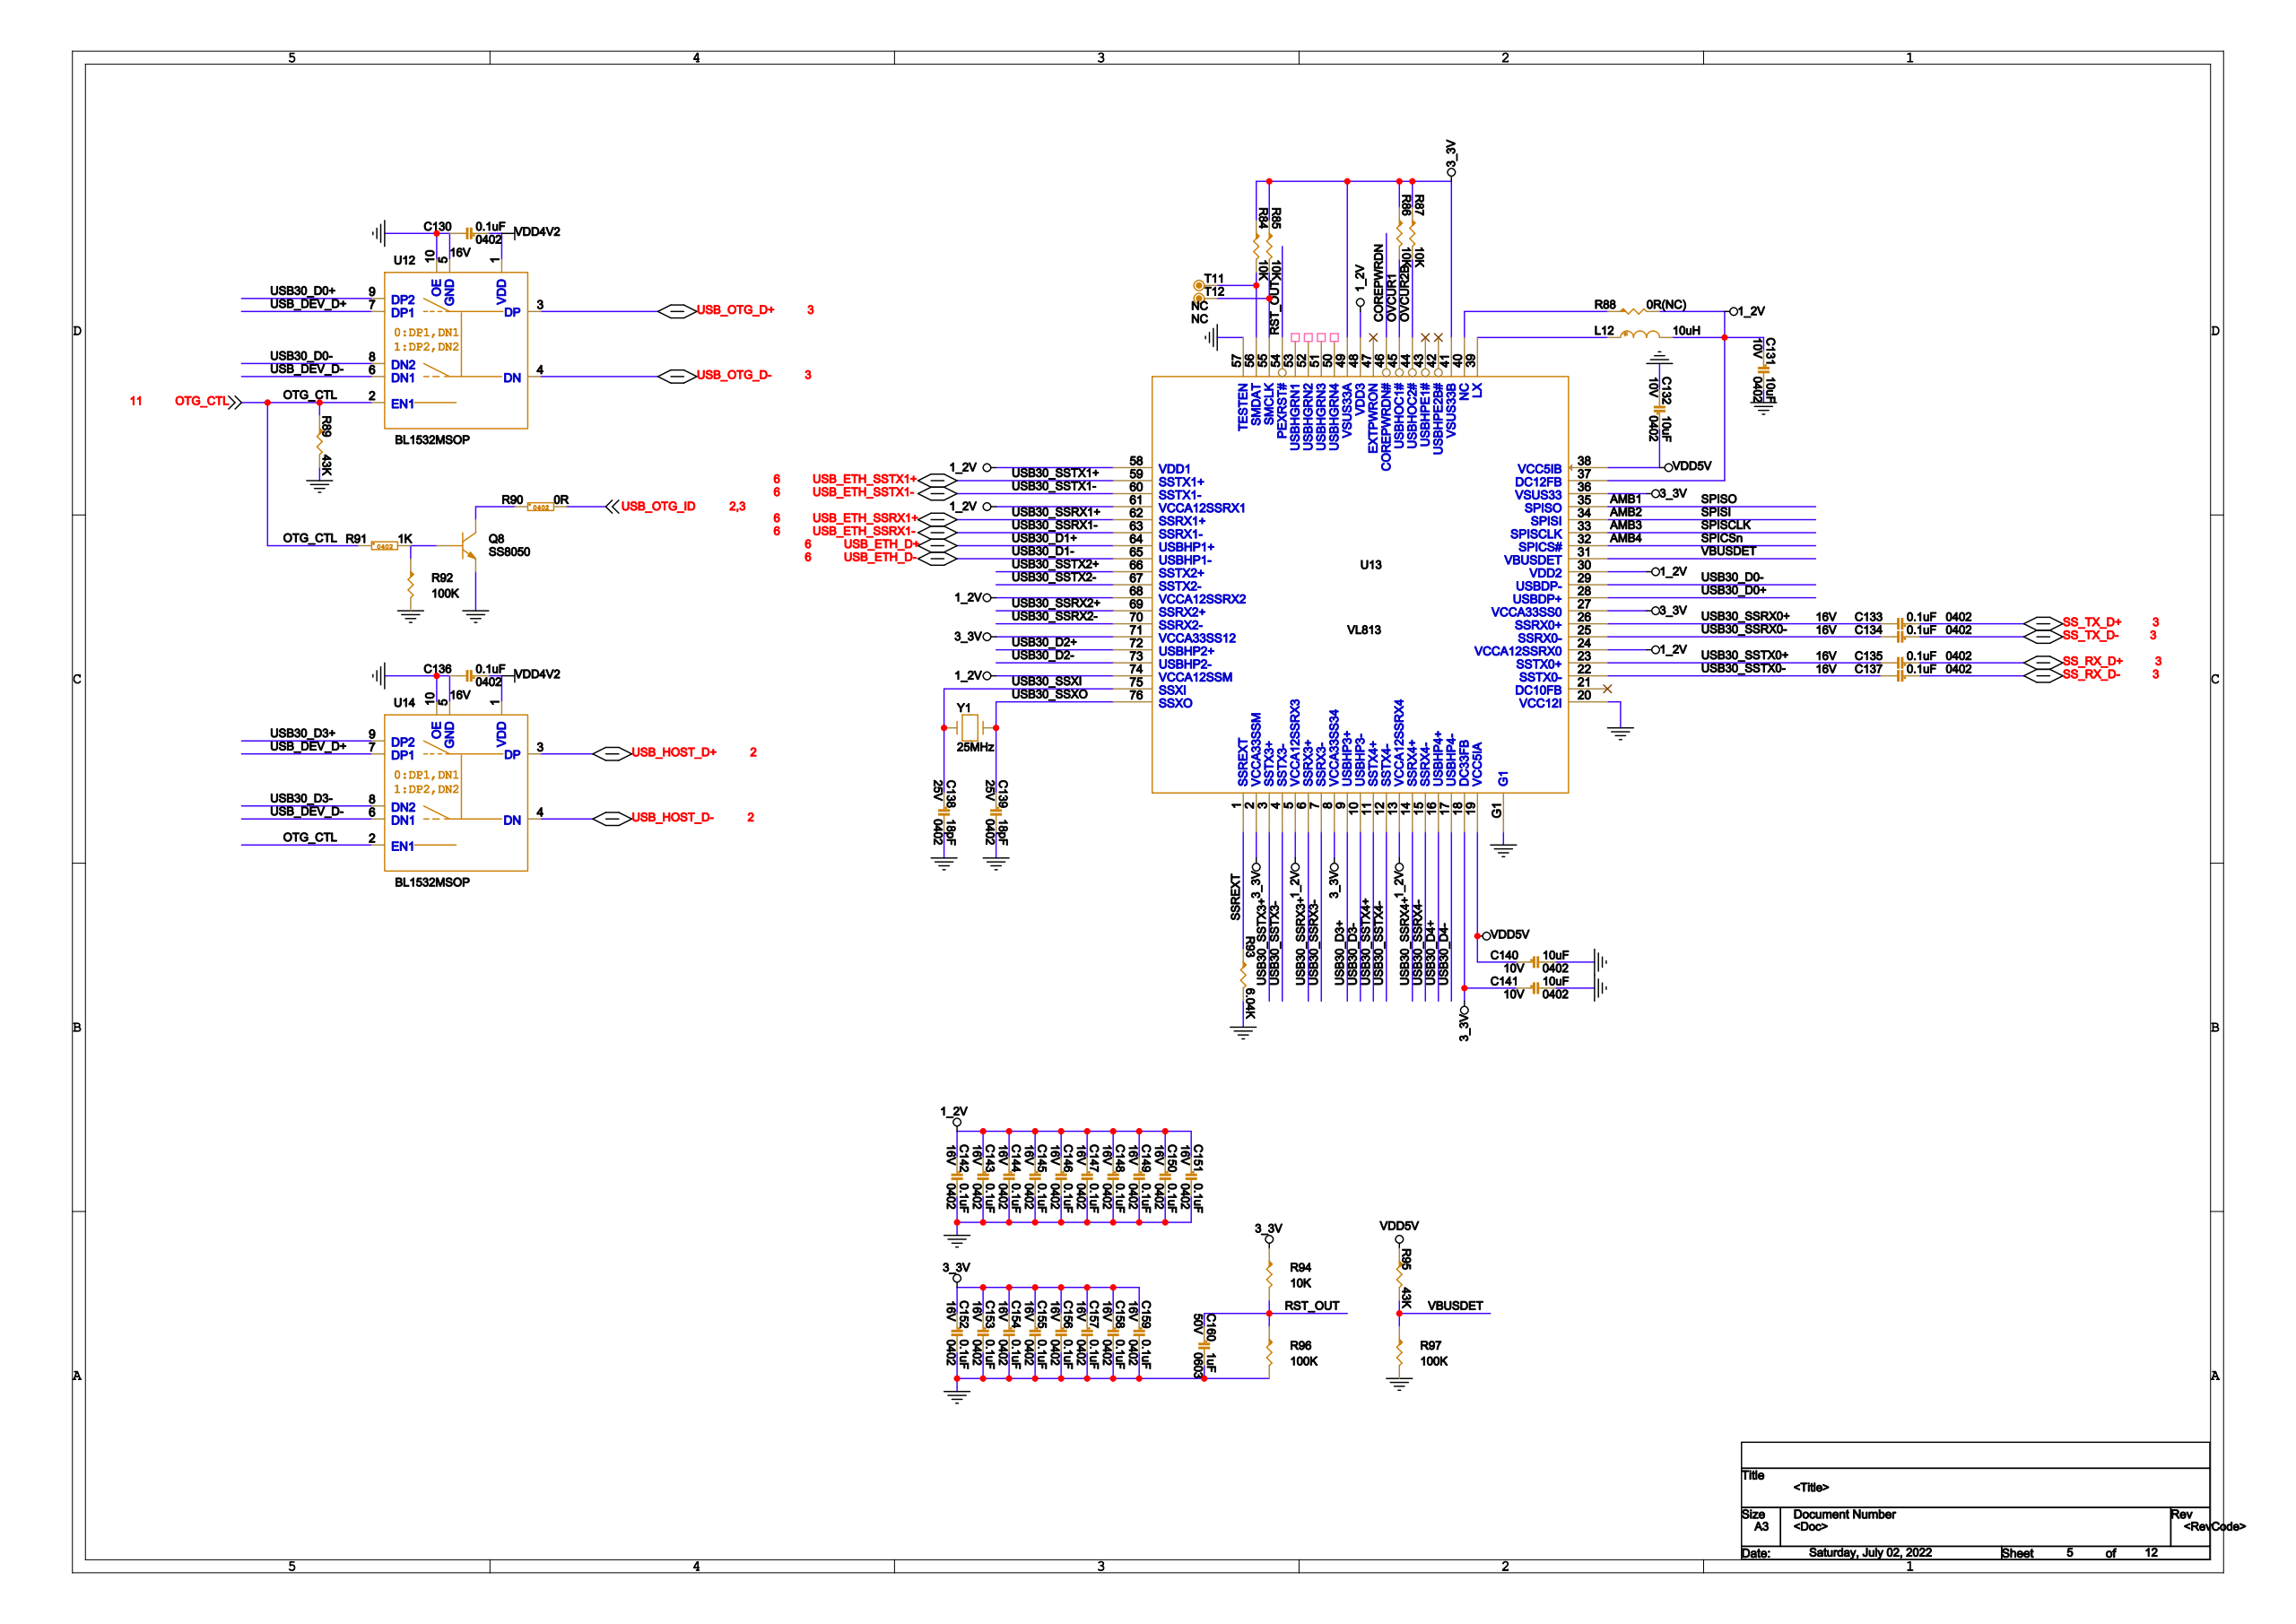Circuit board | Cadence Allegro | 970 parts | 627 nets | one sheet of the schematic
Parts on this sheet (reference | value | footprint):
C130 | 0.1uF | C0402
C131 | 10uF | C0402
C132 | 10uF | C0402
C133 | 0.1uF | C0402
C134 | 0.1uF | C0402
C135 | 0.1uF | C0402
C136 | 0.1uF | C0402
C137 | 0.1uF | C0402
C138 | 18pF | C0402
C139 | 18pF | C0402
C140 | 10uF | C0402
C141 | 10uF | C0402
C142 | 0.1uF | C0402
C143 | 0.1uF | C0402
C144 | 0.1uF | C0402
C145 | 0.1uF | C0402
C146 | 0.1uF | C0402
C147 | 0.1uF | C0402
C148 | 0.1uF | C0402
C149 | 0.1uF | C0402
C150 | 0.1uF | C0402
C151 | 0.1uF | C0402
C152 | 0.1uF | C0402
C153 | 0.1uF | C0402
C154 | 0.1uF | C0402
C155 | 0.1uF | C0402
C156 | 0.1uF | C0402
C157 | 0.1uF | C0402
C158 | 0.1uF | C0402
C159 | 0.1uF | C0402
C160 | 1uF | C0603
L12 | 10uH | L2520
Q8 | SS8050 | SOT-23
R84 | 10K | R0402
R85 | 10K | R0402
R86 | 10K | R0402
R87 | 10K | R0402
R88 | 0R(NC) | R0402
R89 | 43K | R0402
R90 | 0R | R0402
R91 | 1K | R0402
R92 | 100K | R0402
R93 | 6.04K | R0402
R94 | 10K | R0402
R95 | 43K | R0402
R96 | 100K | R0402
R97 | 100K | R0402
T11 | NC | C035S
T12 | NC | C035S
U12 | BL1532MSOP | MSOP10
U13 | VL813 | QFN_76
U14 | BL1532MSOP | MSOP10
Y1 | 25MHz | X3225
Nets of these parts (net: part-pin ...):
VDD5V: C132-1 C140-1 R95-1 U13-19 U13-38
GND: C130-2 C131-2 C132-2 C136-2 C138-2 C139-2 C140-2 C141-2 C142-2 C143-2 C144-2 C145-2 C146-2 C147-2 C148-2 C149-2 C150-2 C151-2 C152-2 C153-2 C154-2 C155-2 C156-2 C157-2 C158-2 C159-2 C160-2 Q8-2 R89-2 R92-2 R93-2 R96-2 R97-2 U12-5 U12-10 U14-5 U14-10 Y1-2 Y1-4 U13-20 U13-57 U13-G1
VDD4V2: C130-1 C136-1 U12-1 U14-1
USB_HOST_D+: U14-3
USB_HOST_D-: U14-4
N19266744: Q8-3 R90-1
USB_OTG_ID: R90-2
OTG_CTL: R89-1 R91-1 U12-2 U14-2
N19266937: Q8-1 R91-2 R92-1
USB30_SSXI: C138-1 Y1-1 U13-75
USB30_SSXO: C139-1 Y1-3 U13-76
RST_OUT: C160-1 R94-2 R96-1 U13-54
N19250997: L12-1 U13-39
1_2V: C131-1 C142-1 C143-1 C144-1 C145-1 C146-1 C147-1 C148-1 C149-1 C150-1 C151-1 L12-2 R88-2 U13-5 U13-13 U13-24 U13-30 U13-37 U13-48 U13-58 U13-61 U13-68 U13-74
VBUSDET: R95-2 R97-1 U13-31
3_3V: C141-1 C152-1 C153-1 C154-1 C155-1 C156-1 C157-1 C158-1 C159-1 R84-1 R85-1 R86-1 R87-1 R94-1 U13-2 U13-8 U13-18 U13-27 U13-36 U13-41 U13-49 U13-71
N19251738: R84-2 T11-1 U13-56
N19251745: R85-2 T12-1 U13-55
OVCUR1: R86-2 U13-45
OVCUR2B: R87-2 U13-44
SSREXT: R93-1 U13-1
N19251086: R88-1 U13-40
USB_OTG_D-: U12-4
USB_DEV_D-: U12-6 U14-6
USB30_D0-: U12-8 U13-29
USB_OTG_D+: U12-3
USB_DEV_D+: U12-7 U14-7
USB30_D0+: U12-9 U13-28
USB30_D3-: U14-8 U13-10
USB30_D3+: U14-9 U13-9
USB_ETH_D+: U13-64
COREPWRDN: U13-46
AMB4: U13-32
AMB3: U13-33
AMB2: U13-34
AMB1: U13-35
USB30_SSRX0+: C133-2 U13-26
USB30_SSRX0-: C134-2 U13-25
USB_ETH_SSRX1+: U13-62
USB_ETH_SSRX1-: U13-63
USB30_SSRX2+: U13-69
USB30_SSRX2-: U13-70
USB30_SSRX3+: U13-6
USB30_SSRX3-: U13-7
USB30_SSRX4+: U13-14
USB30_SSRX4-: U13-15
USB30_SSTX0+: C135-2 U13-23
USB30_SSTX0-: C137-2 U13-22
USB_ETH_SSTX1+: U13-59
USB_ETH_SSTX1-: U13-60
USB30_SSTX2+: U13-66
USB30_SSTX2-: U13-67
USB30_SSTX3+: U13-3
USB30_SSTX3-: U13-4
USB30_SSTX4+: U13-11
USB30_SSTX4-: U13-12
USB30_D2+: U13-72
USB30_D2-: U13-73
USB30_D4+: U13-16
USB30_D4-: U13-17
SS_RX_D-: C137-1
SS_RX_D+: C135-1
SS_TX_D-: C134-1
SS_TX_D+: C133-1